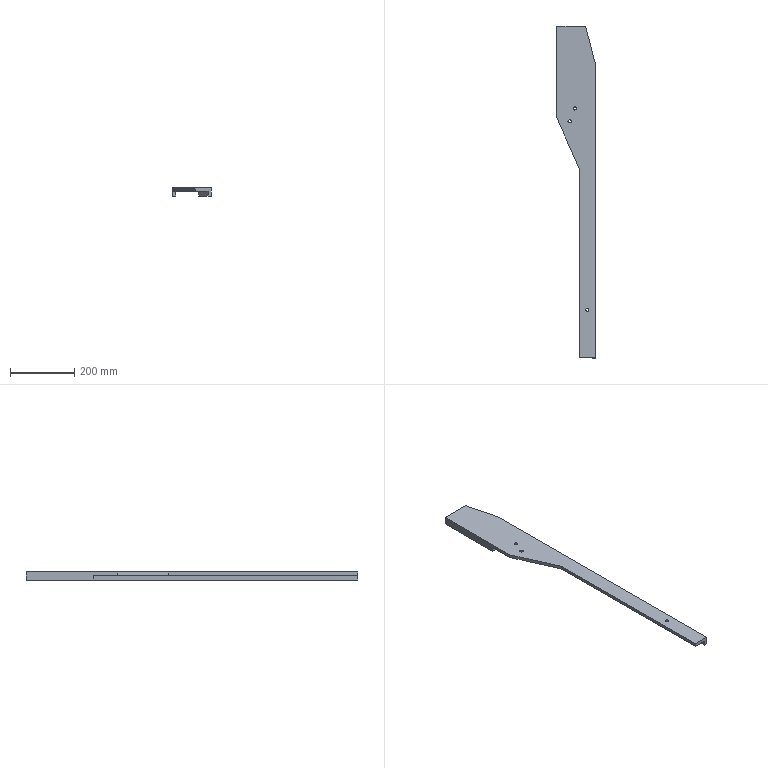Part | STEP file | 1 solid | 22 faces | box 120 x 1034 x 25 mm | volume 939315 mm3 | plane 16 | cylinder 6 | commonest cylinder face diameters 10 x6